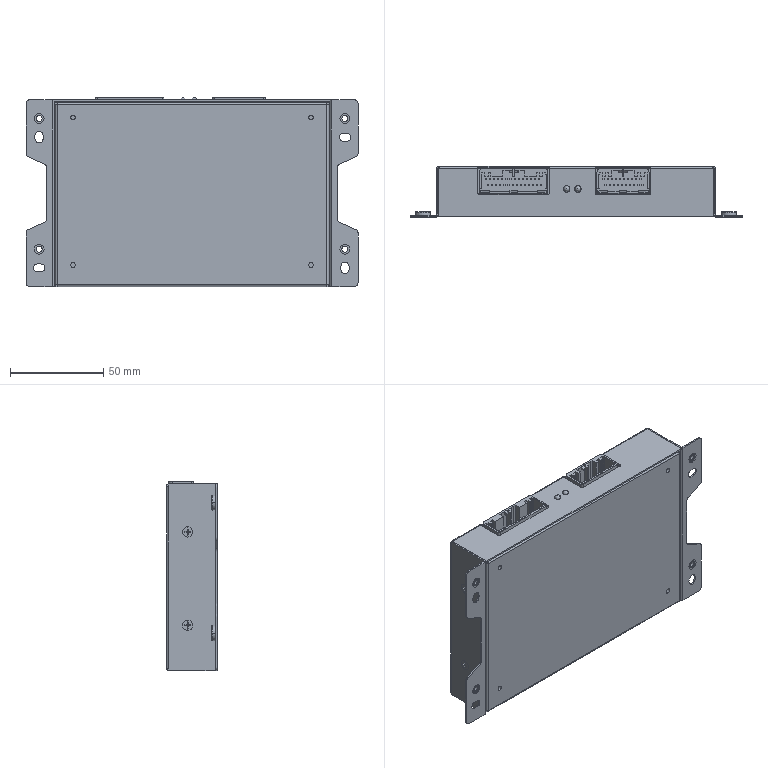Part | SolidWorks | 21 solids | 2981 faces | box 177.9 x 27.2 x 101.3 mm | volume 74977 mm3 | cylinder 1627 | plane 1300 | cone 30 | spline 22 | sphere 2 | commonest cylinder face diameters 0.305 x890 0.889 x112 1 x107 0.6 x64 0.381 x40 0.36 x28